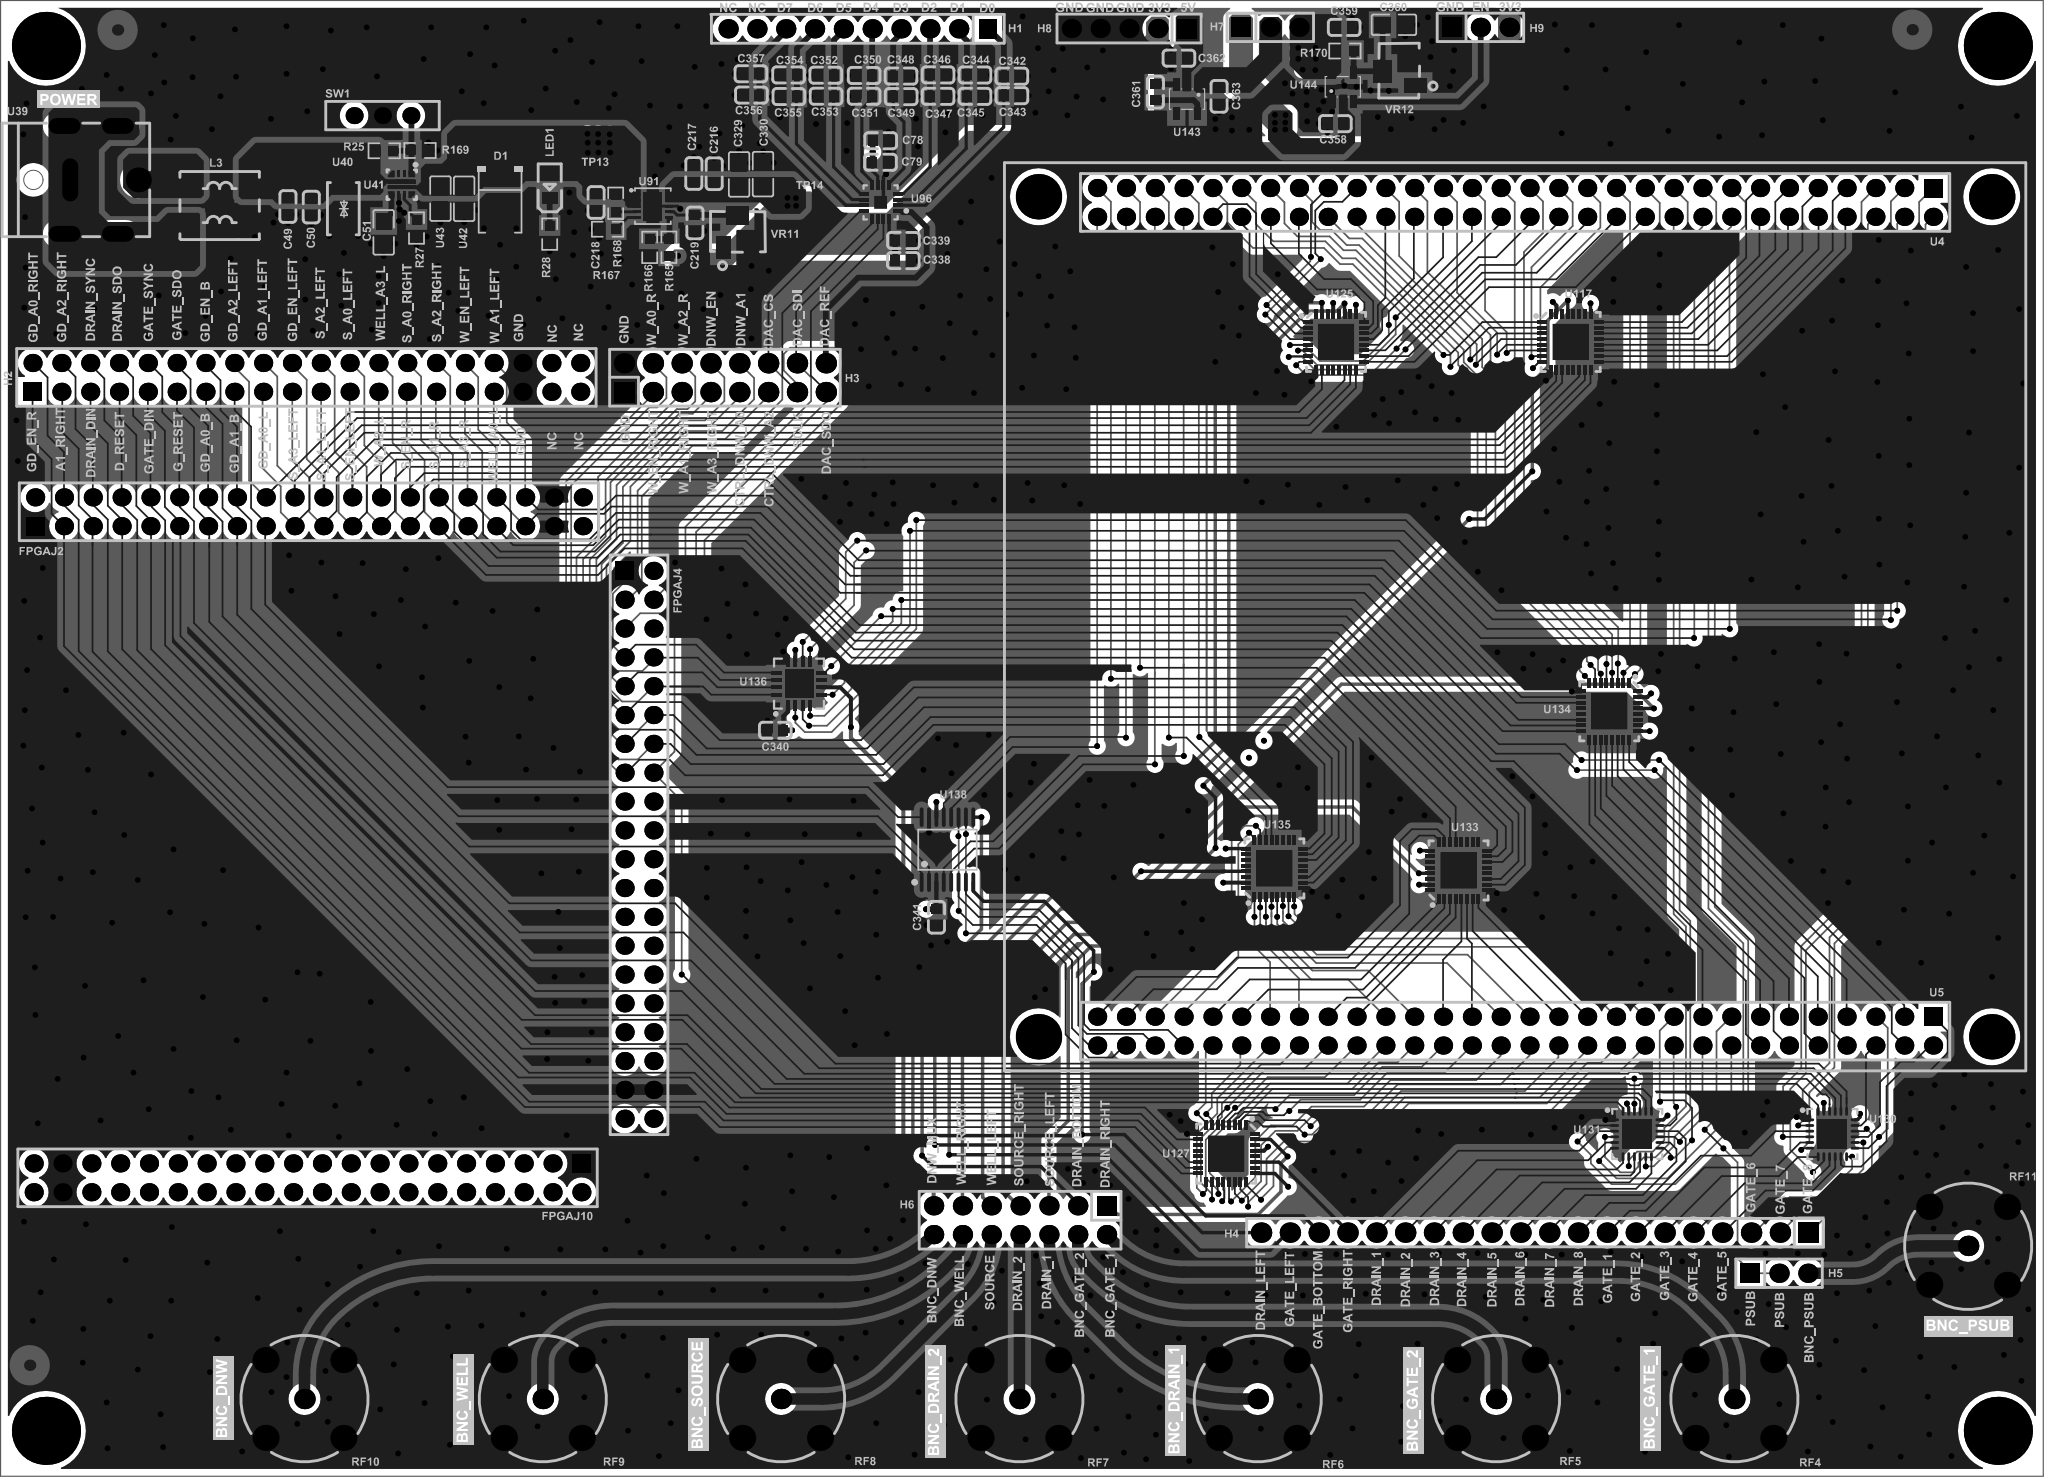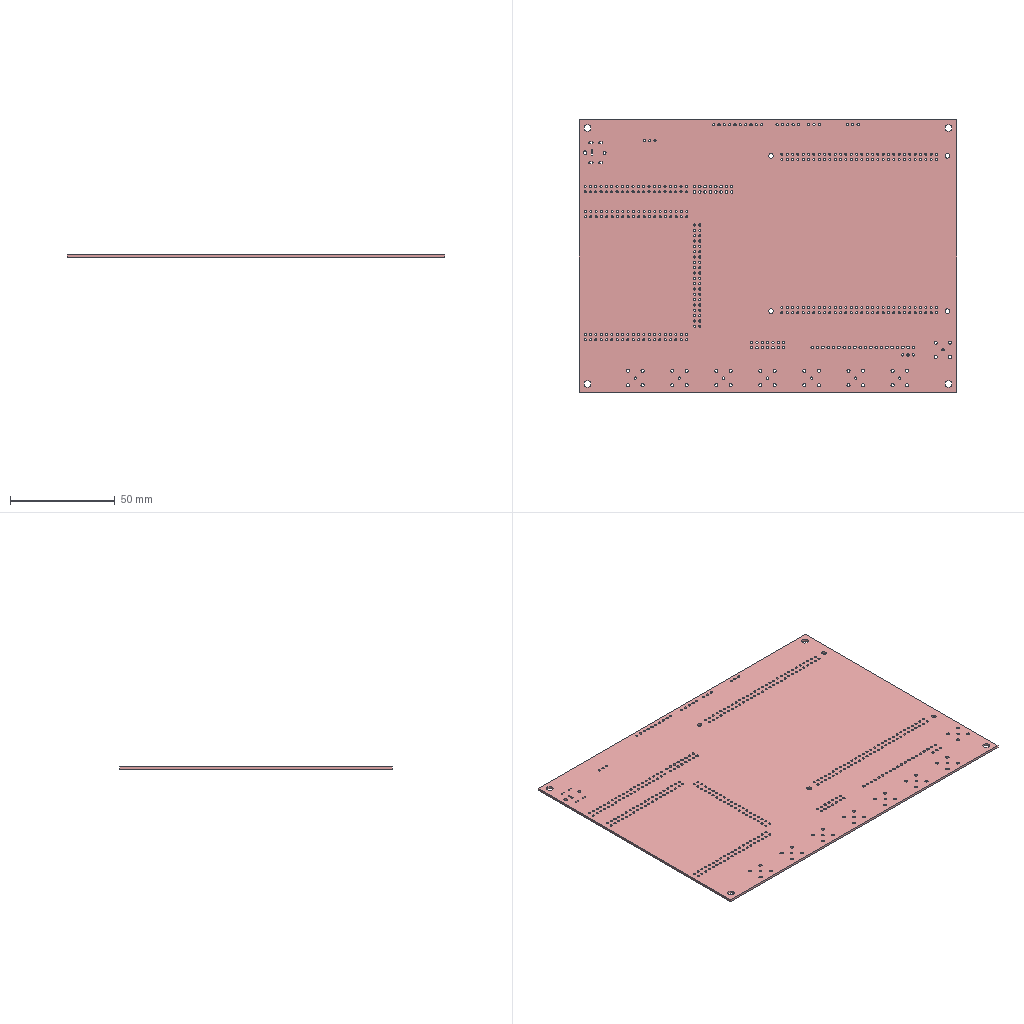Circuit board layout | Altium Designer | box 180 x 130 x 1.1 mm
Layer stack:
# Altium Designer layer stack of  (unit mm; dielectric type: 0 none, 1 core, 2 prepreg, 3 surface material)
index,name,kind,layer,copper_thickness_mm,dielectric_type,dielectric_thickness_mm,dielectric_material,dielectric_constant
0,Top Paste,other,,,,,,
1,Top Overlay,other,,,,,,
2,Top Solder,dielectric,,,3,0.0102,Solder Resist,3.5
3,Top Layer,copper,Top Layer,0.0356,,,,
4,Dielectric1,dielectric,,,1,0.32,FR-4,4.8
5,GND,copper,GND,0.0356,,,,
6,Dielectric2,dielectric,,,2,0.32,FR-4,4.8
7,POWER,copper,POWER,0.0356,,,,
8,Dielectric3,dielectric,,,1,0.32,FR-4,4.8
9,Bottom Layer,copper,Bottom Layer,0.0356,,,,
10,Bottom Solder,dielectric,,,3,0.0102,Solder Resist,3.5
11,Bottom Overlay,other,,,,,,
12,Bottom Paste,other,,,,,,
# drill layer pairs: low layer,high layer
drill_pair,Top Layer,Bottom Layer
Part placement:
Designator,Comment,Layer,Footprint,Center-X(mm),Center-Y(mm),Rotation
TP14,3P3V,TopLayer,Test-Point-0.5mm,69.164,113.716,90
TP13,5V,TopLayer,Test-Point-0.5mm,52.476,114.783,90
H6,PZ254V-12-14P,TopLayer,HDR-TH_14P-P2.54-V-M-R2-C7-S2.54,89.84,22.555,180
H4,PZ254-1-20-W-8.5,TopLayer,HDR-TH_20P-P2.54-V-M-1,135.204,21.463,180
H3,PZ254V-12-16P,TopLayer,HDR-TH_16P-P2.54-V-M-R2-C8-S2.54,63.83,96.774,360
H2,PZ254-2-20-W-8.5,TopLayer,HDR-TH_40P-P2.54-V-F-R2-C20-S2.54,26.949,96.799,360
VR11,,TopLayer,RES-ADJ-SMD_3224W,64.922,109.652,0
U136,ADG1408YCPZ-REEL7,TopLayer,LFCSP-16_L4.0-W4.0-P0.65-BL-EP,70.358,69.825,360
U135,ADG1406BCPZ-REEL7,TopLayer,LFCSP-32_L5.0-W5.0-P0.50-TL-EP3.1,112.243,53.543,90
U134,ADG1406BCPZ-REEL7,TopLayer,LFCSP-32_L5.0-W5.0-P0.50-TL-EP3.1,141.757,67.386,270
U133,ADG1406BCPZ-REEL7,TopLayer,LFCSP-32_L5.0-W5.0-P0.50-TL-EP3.1,128.473,53.365,90
U131,ADG1414BCPZ-REEL7,TopLayer,LFCSP-24_L4.0-W4.0-P0.50-BL-EP,144.221,30.15,270
U130,ADG1414BCPZ-REEL7,TopLayer,LFCSP-24_L4.0-W4.0-P0.50-BL-EP,161.417,30.15,270
U127,ADG1407BCPZ-REEL7,TopLayer,LFCSP-32_L5.0-W5.0-P0.50-BL-EP3.1,108.001,28.423,180
U125,ADG1407BCPZ-REEL7,TopLayer,LFCSP-32_L5.0-W5.0-P0.50-BL-EP3.1,117.678,99.924,270
U117,ADG1406BCPZ-REEL7,TopLayer,LFCSP-32_L5.0-W5.0-P0.50-TL-EP3.1,138.354,99.924,360
U96,DAC80508ZRTER,TopLayer,WQFN-16_L3.0-W3.0-P0.50-TL-EP0.8,77.546,112.217,180
U91,LT3045IDD#PBF,TopLayer,DFN-10_L3.0-W3.0-P0.50-BL-EP-3,57.48,111.887,270
U43,22uF,TopLayer,C0805,38.76,112.547,90
U42,22uF,TopLayer,C0805,40.85,112.536,90
U41,TPS259472ARPWR,TopLayer,VQFN-10_L2.0-W2.0-P0.45-TL,35.331,113.817,270
U40,SMAJ12CA,TopLayer,SMA_L4.3-W2.7-LS5.1-BI,30.251,111.658,90
U39,HX DC007B-2.5,TopLayer,DC-IN-TH_HX-DC007B-2.5,8.89,114.198,0
U5,ZX-PM2.54-2-30PY,TopLayer,HDR-TH_60P-P2.54-V-F-R2-C30-S2.54,133.46,39.212,180
U4,ZX-PM2.54-2-30PY,TopLayer,HDR-TH_60P-P2.54-V-F-R2-C30-S2.54,133.46,112.212,180
SW1,K3-1204D,TopLayer,SW-TH_K3-1204D,33.655,119.863,0
RF10,DOSIN-801-0057,TopLayer,ANT-TH_DOSIN-801-0057,26.781,6.807,180
RF9,DOSIN-801-0057,TopLayer,ANT-TH_DOSIN-801-0057,47.781,6.807,180
RF8,DOSIN-801-0057,TopLayer,ANT-TH_DOSIN-801-0057,68.781,6.807,180
RF7,DOSIN-801-0057,TopLayer,ANT-TH_DOSIN-801-0057,89.781,6.807,180
RF6,DOSIN-801-0057,TopLayer,ANT-TH_DOSIN-801-0057,110.781,6.807,180
RF5,DOSIN-801-0057,TopLayer,ANT-TH_DOSIN-801-0057,131.781,6.807,180
RF4,DOSIN-801-0057,TopLayer,ANT-TH_DOSIN-801-0057,152.781,6.807,180
R168,,TopLayer,R0603,54.204,112.141,90
R167,,TopLayer,R0603,53.492,109.855,0
R166,,TopLayer,R0603,57.201,108.255,90
R165,,TopLayer,R0603,58.893,108.266,270
R28,,TopLayer,R0603,48.387,109.423,90
R27,,TopLayer,R0603,36.652,109.957,270
R25,,TopLayer,R0603,33.807,116.764,360
LED1,NCD0805G1,TopLayer,LED0805-R-RD,48.387,113.614,90
H1,PZ254V-11-10P,TopLayer,HDR-TH_10P-P2.54-V-M,75.54,127.508,180
FPGAJ10,2.54-2*20,TopLayer,HDR-TH_40P-P2.54-V-F-R2-C20-S2.54,27.051,26.289,180
FPGAJ4,2.54-2*20,TopLayer,HDR-TH_40P-P2.54-V-F-R2-C20-S2.54,56.261,55.626,270
FPGAJ2,2.54-2*20,TopLayer,HDR-TH_40P-P2.54-V-F-R2-C20-S2.54,27.178,84.963,0
D1,VS-10BQ015HM3/5BT,TopLayer,SMB_L4.6-W3.6-LS5.3-RD,44.018,112.293,270
C357,10uF,TopLayer,C0603,66.126,123.543,360
C356,100nF,TopLayer,C0603,66.171,121.666,360
C355,10uF,TopLayer,C0603,69.473,121.539,360
C354,100nF,TopLayer,C0603,69.447,123.441,360
C353,10uF,TopLayer,C0603,72.749,121.564,360
C352,100nF,TopLayer,C0603,72.724,123.419,360
C351,10uF,TopLayer,C0603,76.102,121.564,360
C350,100nF,TopLayer,C0603,76.102,123.393,360
C349,10uF,TopLayer,C0603,79.353,121.539,180
C348,100nF,TopLayer,C0603,79.341,123.35,180
C347,10uF,TopLayer,C0603,82.605,121.564,180
C346,100nF,TopLayer,C0603,82.605,123.452,180
C345,10uF,TopLayer,C0603,85.856,121.564,180
C344,100nF,TopLayer,C0603,85.856,123.444,180
C343,10uF,TopLayer,C0603,89.113,121.623,180
C342,100nF,TopLayer,C0603,89.107,123.342,180
C341,10uF,TopLayer,C0603,82.474,49.251,90
C340,100nF,TopLayer,C0603,68.275,65.71,360
C339,10uF,TopLayer,C0603,79.553,108.864,180
C338,100nF,TopLayer,C0603,79.54,107.096,180
C330,10uF,TopLayer,C0805,67.183,114.706,270
C329,100nF,TopLayer,C0805,65.078,114.681,270
C219,4.7uF,TopLayer,C0603,61.189,110.414,90
C218,22uF,TopLayer,C0603,52.476,112.217,90
C217,22uF,TopLayer,C0603,61.087,114.757,270
C216,22uF,TopLayer,C0603,62.88,114.735,270
C79,10uF,TopLayer,C0603,77.527,115.757,180
C78,100nF,TopLayer,C0603,77.546,117.653,180
C51,10nF,TopLayer,C0805,33.757,109.576,90
C50,100nF,TopLayer,C0603,27.381,111.811,90
C49,100nF,TopLayer,C0603,25.324,111.862,90
C358,2.2uF,TopLayer,C0603,117.627,119.151,360
C359,2.2uF,TopLayer,C0603,118.389,127.635,180
C360,10nF,TopLayer,C0805,122.784,127.864,180
C361,1uF,TopLayer,C0603,101.761,121.923,270
C362,1uF,TopLayer,C0603,103.844,124.921,360
C363,1uF,TopLayer,C0603,107.374,121.568,90
H7,PZ254V-11-03P,TopLayer,HDR-TH_3P-P2.54-V-M,111.887,127.635,360
H8,PZ254V-11-05P,TopLayer,HDR-TH_5P-P2.54-V-M,99.441,127.533,180
H9,PZ254V-11-03P,TopLayer,HDR-TH_3P-P2.54-V-M,130.404,127.635,360
L3,PCAQ7060MW-301,TopLayer,FILTER-SMD_4P-L7.0-W6.0-BL,19.304,111.938,270
R169,,TopLayer,R0603,36.957,116.789,360
R170,,TopLayer,R0603,118.466,125.552,180
U138,ADG1409YRUZ-REEL7,TopLayer,TSSOP-16_L5.0-W4.4-P0.65-LS6.4-BL,83.439,55.194,360
U143,TPS60403DBVR,TopLayer,SOT-23-5_L3.0-W1.7-P0.95-LS2.8-BR,104.549,121.314,90
U144,TPS72301DBVR,TopLayer,SOT-23-5_L3.0-W1.7-P0.95-LS2.8-BR,118.277,122.403,270
VR12,,TopLayer,RES-ADJ-SMD_3224W,123.215,123.774,90
RF11,DOSIN-801-0057,TopLayer,ANT-TH_DOSIN-801-0057,173.38,20.295,0
H5,PZ254V-11-03P,TopLayer,HDR-TH_3P-P2.54-V-M,156.718,17.882,360
Pad and via stacks:
# Altium Designer via and pad stacks of  (unit mm). Each distinct definition once, with the count of objects using it.
# via: kind,start_layer,end_layer,hole_mm,diameter_mm,mode(0 simple;1 top-mid-bottom;2 full stack),diameter_per_layer,count,example_net
# pad: kind,layer,hole_mm,hole_type(0 round;1 square;2 slot),plating,top_size,top_shape(1 round;2 rect;3 octagon;9 rounded rect),mid_size,bottom_size,mode,footprint,size_per_layer,count,example
pad,Multi-Layer,1.1,0,plated,1.7x1.7,1,1.7x1.7,1.7x1.7,0,HDR-TH_10P-P2.54-V-M,,9,H1.10
pad,Multi-Layer,1.1,0,plated,1.575x1.7,2,1.575x1.7,1.575x1.7,0,HDR-TH_10P-P2.54-V-M,,1,H1.1
pad,Multi-Layer,1.1,0,plated,1.8x1.8,1,1.8x1.8,1.8x1.8,0,ANT-TH_DOSIN-801-0057,,8,RF10.1
pad,Multi-Layer,1.5,0,plated,2.3x2.3,1,2.3x2.3,2.3x2.3,0,ANT-TH_DOSIN-801-0057,,32,RF10.2
pad,Multi-Layer,1,0,plated,1.5x1.5,1,1.5x1.5,1.5x1.5,0,SW-TH_K3-1204D,,3,SW1.3
pad,Multi-Layer,1,0,plated,1.6x1.6,2,1.6x1.6,1.6x1.6,0,HDR-TH_60P-P2.54-V-F-R2-C30-S2.54,,2,U5.1
pad,Multi-Layer,1,0,plated,1.6x1.6,1,1.6x1.6,1.6x1.6,0,HDR-TH_60P-P2.54-V-F-R2-C30-S2.54,,118,U5.2
pad,Multi-Layer,1.4,0,plated,2.2x2.2,1,2.2x2.2,2.2x2.2,0,DC-IN-TH_HX-DC007B-2.5,,1,U39.1
pad,Multi-Layer,0.8,2,plated,1.4x3.8,1,1.4x3.8,1.4x3.8,0,DC-IN-TH_HX-DC007B-2.5,,1,U39.2
pad,Multi-Layer,0.8,2,plated,1.4x2.8,1,1.4x2.8,1.4x2.8,0,DC-IN-TH_HX-DC007B-2.5,,4,U39.3
pad,Multi-Layer,1,0,plated,1.6x1.6,2,1.6x1.6,1.6x1.6,0,HDR-TH_40P-P2.54-V-F-R2-C20-S2.54,,4,H2.1
pad,Multi-Layer,1,0,plated,1.6x1.6,1,1.6x1.6,1.6x1.6,0,HDR-TH_40P-P2.54-V-F-R2-C20-S2.54,,156,H2.2
pad,Multi-Layer,1.2,0,plated,1.8x1.8,2,1.8x1.8,1.8x1.8,0,HDR-TH_16P-P2.54-V-M-R2-C8-S2.54,,1,H3.1
pad,Multi-Layer,1.2,0,plated,1.8x1.8,1,1.8x1.8,1.8x1.8,0,HDR-TH_16P-P2.54-V-M-R2-C8-S2.54,,15,H3.2
pad,Multi-Layer,1.2,0,plated,1.8x1.8,1,1.8x1.8,1.8x1.8,0,HDR-TH_20P-P2.54-V-M-1,,19,H4.20
pad,Multi-Layer,1.2,0,plated,1.8x1.8,2,1.8x1.8,1.8x1.8,0,HDR-TH_20P-P2.54-V-M-1,,1,H4.1
pad,Multi-Layer,1.1,0,plated,1.7x1.7,1,1.7x1.7,1.7x1.7,0,HDR-TH_14P-P2.54-V-M-R2-C7-S2.54,,13,H6.14
pad,Multi-Layer,1.1,0,plated,1.7x1.7,2,1.7x1.7,1.7x1.7,0,HDR-TH_14P-P2.54-V-M-R2-C7-S2.54,,1,H6.1
pad,Multi-Layer,3.2,0,plated,6x6,1,6x6,6x6,0,,,4,0
pad,Multi-Layer,2.2,0,plated,4x4,1,4x4,4x4,0,,,4,0
pad,Multi-Layer,1.1,0,plated,1.7x1.7,1,1.7x1.7,1.7x1.7,0,HDR-TH_5P-P2.54-V-M,,4,H8.5
pad,Multi-Layer,1.1,0,plated,1.7x1.7,2,1.7x1.7,1.7x1.7,0,HDR-TH_5P-P2.54-V-M,,1,H8.1
pad,Multi-Layer,1.1,0,plated,1.7x1.7,1,1.7x1.7,1.7x1.7,0,HDR-TH_3P-P2.54-V-M,,6,H9.3
pad,Multi-Layer,1.1,0,plated,1.7x1.7,2,1.7x1.7,1.7x1.7,0,HDR-TH_3P-P2.54-V-M,,3,H9.1
pad,Top Layer,0,0,plated,1x1,1,1x1,1x1,0,,,3,MARK
pad,Top Layer,0,0,plated,0.8x0.9,2,0.8x0.9,0.8x0.9,0,C0603,,66,C357.2
pad,Top Layer,0,0,plated,2.047x2.192,2,2.047x2.192,2.047x2.192,0,SMB_L4.6-W3.6-LS5.3-RD,,2,D1.2
pad,Top Layer,0,0,plated,1x1.399,2,1x1.399,1x1.399,0,LED0805-R-RD,,2,LED1.2
pad,Top Layer,0,0,plated,0.8065x0.864,2,0.8065x0.864,0.8065x0.864,0,R0603,,18,R168.2
pad,Top Layer,0,0,plated,2.1x1.8,2,2.1x1.8,2.1x1.8,0,SMA_L4.3-W2.7-LS5.1-BI,,2,U40.2
pad,Top Layer,0,0,plated,0.36x0.36,1,0.36x0.36,0.36x0.36,0,VQFN-10_L2.0-W2.0-P0.45-TL,,4,U41.1
pad,Top Layer,0,0,plated,0.3x2.4,2,0.3x2.4,0.3x2.4,0,VQFN-10_L2.0-W2.0-P0.45-TL,,2,U41.5
pad,Top Layer,0,0,plated,0.25x0.6,2,0.25x0.6,0.25x0.6,0,VQFN-10_L2.0-W2.0-P0.45-TL,,4,U41.2
pad,Top Layer,0,0,plated,1.41x1.35,2,1.41x1.35,1.41x1.35,0,C0805,,12,U43.2
pad,Top Layer,0,0,plated,0.25x0.65,2,0.25x0.65,0.25x0.65,0,DFN-10_L3.0-W3.0-P0.50-BL-EP-3,,10,U91.1
pad,Top Layer,0,0,plated,2.5x1.6,2,2.5x1.6,2.5x1.6,0,DFN-10_L3.0-W3.0-P0.50-BL-EP-3,,1,U91.11
pad,Top Layer,0,0,plated,0.8x0.8,2,0.8x0.8,0.8x0.8,0,WQFN-16_L3.0-W3.0-P0.50-TL-EP0.8,,1,U96.17
pad,Top Layer,0,0,plated,0.28x0.85,2,0.28x0.85,0.28x0.85,0,WQFN-16_L3.0-W3.0-P0.50-TL-EP0.8,,16,U96.16
pad,Top Layer,0,0,plated,0.8x0.2997,2,0.8x0.2997,0.8x0.2997,0,LFCSP-32_L5.0-W5.0-P0.50-BL-EP3.1,,32,U127.32
pad,Top Layer,0,0,plated,0.3x0.8,2,0.3x0.8,0.3x0.8,0,LFCSP-32_L5.0-W5.0-P0.50-BL-EP3.1,,32,U127.24
pad,Top Layer,0,0,plated,3.1x3.1,2,3.1x3.1,3.1x3.1,0,LFCSP-32_L5.0-W5.0-P0.50-BL-EP3.1,,2,U127.33
pad,Top Layer,0,0,plated,0.8x0.25,1,0.8x0.25,0.8x0.25,0,LFCSP-24_L4.0-W4.0-P0.50-BL-EP,,24,U131.24
pad,Top Layer,0,0,plated,0.25x0.8,1,0.25x0.8,0.25x0.8,0,LFCSP-24_L4.0-W4.0-P0.50-BL-EP,,24,U131.18
pad,Top Layer,0,0,plated,2.6x2.6,2,2.6x2.6,2.6x2.6,0,LFCSP-24_L4.0-W4.0-P0.50-BL-EP,,2,U131.25
pad,Top Layer,0,0,plated,0.8x0.2997,2,0.8x0.2997,0.8x0.2997,0,LFCSP-32_L5.0-W5.0-P0.50-TL-EP3.1,,64,U135.32
pad,Top Layer,0,0,plated,0.3x0.8,2,0.3x0.8,0.3x0.8,0,LFCSP-32_L5.0-W5.0-P0.50-TL-EP3.1,,64,U135.24
pad,Top Layer,0,0,plated,3.1x3.1,2,3.1x3.1,3.1x3.1,0,LFCSP-32_L5.0-W5.0-P0.50-TL-EP3.1,,4,U135.33
pad,Top Layer,0,0,plated,2.5x2.5,2,2.5x2.5,2.5x2.5,0,LFCSP-16_L4.0-W4.0-P0.65-BL-EP,,1,U136.17
pad,Top Layer,0,0,plated,0.35x0.9,2,0.35x0.9,0.35x0.9,0,LFCSP-16_L4.0-W4.0-P0.65-BL-EP,,16,U136.1
pad,Top Layer,0,0,plated,2x1.3,2,2x1.3,2x1.3,0,RES-ADJ-SMD_3224W,,4,VR11.1
pad,Top Layer,0,0,plated,1.6x2,2,1.6x2,1.6x2,0,RES-ADJ-SMD_3224W,,2,VR11.2
pad,Top Layer,0,0,plated,1x1,1,1x1,1x1,0,Test-Point-0.5mm,,2,TP14.1
pad,Top Layer,0,0,plated,1.1x0.6,2,1.1x0.6,1.1x0.6,0,SOT-23-5_L3.0-W1.7-P0.95-LS2.8-BR,,10,U144.5
pad,Top Layer,0,0,plated,2.6x1.501,2,2.6x1.501,2.6x1.501,0,FILTER-SMD_4P-L7.0-W6.0-BL,,4,L3.4
pad,Top Layer,0,0,plated,0.343x1.732,1,0.343x1.732,0.343x1.732,0,TSSOP-16_L5.0-W4.4-P0.65-LS6.4-BL,,16,U138.9
via,Top Layer,Bottom Layer,0.3048,0.508,0,,1291,GND
Copper pours:
name,layer,net,type(0 solid;1 hatched;2 none)
Bottom Layer-No Net,Top Layer,GND,0
Bottom Layer-No Net,Top Layer,3P3V,0
Bottom Layer-No Net,Top Layer,NetC358_2,0
Bottom Layer-No Net,Top Layer,5V_NEG,0
Bottom Layer-No Net,Top Layer,NetC363_2,0
Bottom Layer-No Net,Top Layer,5V,0
Bottom Layer-No Net,Top Layer,5V,0
Bottom Layer-No Net,Top Layer,NetC49_2,0
Bottom Layer-No Net,Top Layer,NetL3_2,0
Bottom Layer-No Net,Top Layer,NetL3_1,0
Bottom Layer-No Net,Bottom Layer,GND,0
Bottom Layer-No Net,Bottom Layer,3P3V,0
Bottom Layer-No Net,Bottom Layer,NetC358_2,0
Design rules, without the lines most boards share:
# Altium Designer design rules of  (exported by Altium Designer, unit mm)
# columns: name | kind | enabled | priority | scope1 | scope2 | descriptor | typed fields (field=value)
Clearance_2 | 0 | enabled | 1 | haspad('free-mark') | All | Clearance Constraint (Gap=50mil) (haspad('free-mark')),(All) | gap=1.27
Clearance_1 | 0 | enabled | 2 | inpolygon | All | Clearance Constraint (Gap=6mil) (inpolygon),(All) | gap=0.1524
Clearance | 0 | enabled | 3 | All | All | Clearance Constraint (Gap=6mil) (All),(All) | gap=0.1524
PlaneConnect | 6 | enabled | 1 | All | All | Power Plane Connect Rule(Direct Connect )(Expansion=20mil) (Conductor Width=10mil) (Air Gap=10mil) (Entries=4) (All) | relief_conductor_width=0.254 relief_entries=4 relief_expansion=0.508
PlaneClearance | 12 | enabled | 1 | All | All | Power Plane Clearance (Clearance =6mil) (All) | clearance=0.1524
PolygonConnect | 20 | enabled | 1 | All | All | Polygon Connect Rule(Direct Connect )(Conductor Width=10mil) (Relief Angle=90 Angle) (Entries=4) (Air Gap Width=10mil) (All),(All) | connect_style(0=relief,1=direct,2=none)=1 relief_conductor_width=0.254 relief_entries=4
Width | 2 | enabled | 1 | All | All | Width Constraint (Min=6mil) (Max=40mil) (Preferred=6mil) (All) |
RoutingVias | 11 | enabled | 1 | All | All | Routing Via (MinHoleWidth=12mil) (MaxHoleWidth=12mil) (PreferredHoleWidth=12mil) (MinWidth=20mil) (MaxWidth=20mil) (PreferedWidth=20mil) (All) | via_min_hole=0.3048 via_max_hole=0.3048 via_preferred_diameter=0.508 via_preferred_hole=0.3048
SolderMaskExpansion | 13 | enabled | 1 | All | All | Solder Mask Expansion (Expansion =4mil) (All) | expansion=0.1016
HoleSize | 42 | enabled | 1 | All | All | Hole Size Constraint (Min=1mil) (Max=500mil) (All) |
DiffPairsRouting | 51 | enabled | 1 | All | All | Differential Pairs Uncoupled Length using the Gap Constraints (Min=6mil) (Max=6mil) (Prefered=6mil)  and Width Constraints (Min=15mil) (Max=15mil) (Prefered=15mil) (All) |
HoleToHoleClearance | 52 | enabled | 1 | All | All | Hole To Hole Clearance (Gap=0mil) (All),(All) | gap=0
MinimumSolderMaskSliver | 53 | enabled | 1 | All | All | Minimum Solder Mask Sliver (Gap=0mil) (All),(All) |
SilkscreenOverComponentPads | 54 | enabled | 1 | IsPad | All | Silk To Solder Mask (Clearance=0mil) (IsPad),(All) |
SilkToSilkClearance | 55 | enabled | 1 | All | All | Silk to Silk (Clearance=0mil) (All),(All) |
Classes set for this board:
# Altium Designer classes of  (member kind: 0 net, 1 component, 2 from-to, 3 pad, 4 layer, 5 differential pair, 6 design channel, 7 polygon, 8 structure, 9 xSignal)
# columns: class name | member kind | superclass | members
2_MUX | 1 | no | H4; H6; RF4; RF5; RF6; RF7; RF8; RF9; RF10; U117; U125; U127; U130; U131; U133; U134; U135; U136; H4; H6; U138; RF11; H5;
1_Power | 1 | no | C49; C50; C51; C78; C79; C216; C217; C218; C219; C329; C330; C338; C339; C340; C341; C342; C343; C344; C345; C346; C347; C348; C349; C350; C351; C352; C353; C354; C355; C356; C357; D1; FPGAJ2; FPGAJ4; FPGAJ10; H1; H2; H3; LED1; R25; R27; R28; R165; R166; R167; R168; SW1; TP13; TP14; U4; U5; U39; U40; U41; U42; U43; U91; U96; VR11; TP13; TP14; C358; C359; C360; C361; C362; C363; H7; H8; H9; L3; R169; R170; U143; U144; VR12;